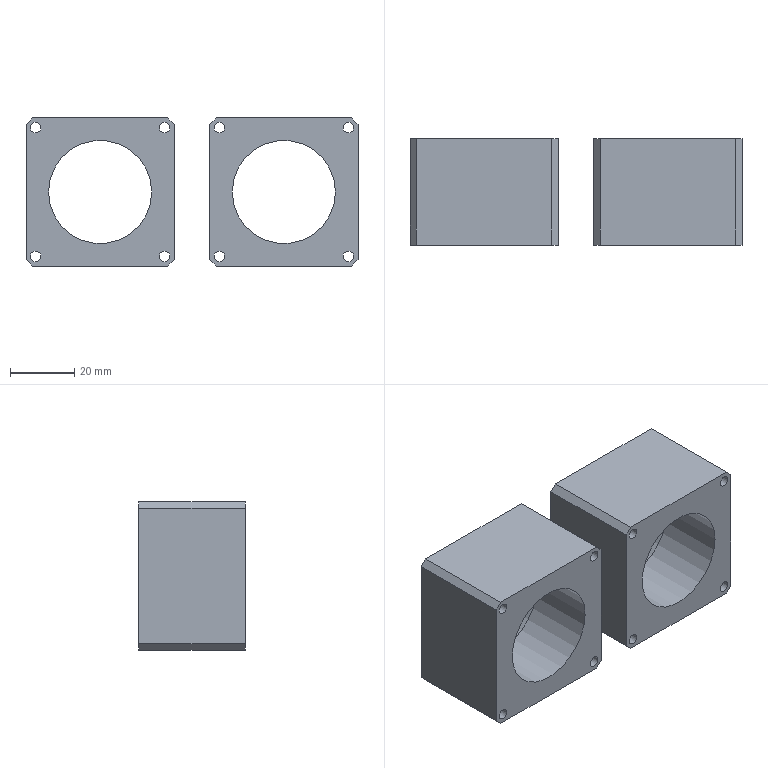CAM job | NX | 3+2 milling, drilling | part box 103 x 33 x 46 mm | stock box 108 x 35 x 51 mm
Tools:
number,name,description,diameter,corner_radius,flute_length,length,flutes
6,D6,平底铣刀-粗,6.0,0.0,25.0,75.0,2
9,D10,平底铣刀-粗,10.0,0.0,35.0,75.0,2
11,D4-J,平底铣刀-精,4.0,0.0,50.0,75.0,2
7,D6-J,平底铣刀-精,6.0,0.0,25.0,75.0,2
10,D10-J,平底铣刀-精,10.0,0.0,35.0,75.0,2
1,D80R0.8飞刀,圆鼻刀-粗,80.0,0.8,50.0,75.0,2
1,D80R0.8飞刀-J,圆鼻刀-精,80.0,0.8,50.0,75.0,2
2,D6倒角刀,倒角刀,6.0,0.0,3.0,25.0,2
20,M3X0.5,丝锥,2.5,0.0,35.0,50.0,2
12,ZT2.6,钻头,2.6,0.0,35.0,50.0,2
13,ZT3.4,钻头,3.4,0.0,35.0,50.0,2
Operations:
program,operation,operation_type,tool,method,geometry_group,spindle_rpm,surface_speed,feed_per_tooth,feed_cut,feed_plunge,cut_length_mm,path_length_mm,cut_time_min,machine_time_min
B,底壁铣飞面一刀开粗_COPY,VolumeBased25DMillingOperation,D80R0.8飞刀,分层开粗-切深K-步距G,W-B,2800.0,703.696,0.5357,3000.0,100.0,1267.165,2586.187,0.4224,0.5543
B,底壁铣飞面一刀精光_COPY,VolumeBased25DMillingOperation,D80R0.8飞刀-J,侧刃精光-切深K-步距G,W-B,4500.0,1130.973,0.1111,1000.0,100.0,210.998,306.998,0.211,0.2206
B,钻倒角_3,Operation,D6倒角刀,METHOD,W-B,8000.0,150.796,0.0625,1000.0,0.0,41.6,439.287,0.0416,0.0814
B,平面去毛刺6X45L_COPY,SurfaceContour,D6倒角刀,爬面_倒角-切深0-步距G,W-B,6500.0,122.519,0.1154,1500.0,100.0,639.96,1426.461,0.4266,0.5053
A,顶面,FaceMilling,D80R0.8飞刀,侧刃精光-切深K-步距G,W-A,4500.0,1385.0,0.1667,1500.0,100.0,197.0,293.0,0.1313,0.1409
A,外形粗_2,VolumeBased25DMillingOperation,D10,METHOD,W-A,8000.0,251.327,0.375,6000.0,80.0,18179.91,18500.41,3.03,3.062
A,型腔铣开粗-中_COPY,CavityMilling,D10,分层开粗-切深K-步距G,W-A,8000.0,251.32,0.25,4000.0,100.0,17009.688,18367.508,4.252,4.439
A,等高往复层切开粗-中_COPY,ZLevelMilling,D6,分层开粗-切深K-步距G,W-A,8000.0,150.792,0.1875,3000.0,100.0,1337.08,7446.112,0.4457,1.057
A,清角D4,ZLevelMilling,D4-J,METHOD,W-A,8000.0,100.531,0.125,2000.0,80.0,2773.694,3173.817,1.387,1.427
A,打点-深0.8,Operation,D6倒角刀,NONE,W-A,8000.0,150.796,0.0312,500.0,90.0,25.2,461.08,0.0504,0.094
A,通孔-M4螺纹底孔,Operation,ZT3.4,NONE,W-A,3000.0,31.102,0.05,300.0,90.0,312.0,965.121,1.04,1.105
A,盲锥孔-M3螺纹底孔,Operation,ZT2.6,NONE,W-A,3000.0,23.562,0.0167,100.0,90.0,84.0,447.614,0.84,0.8764
A,底精_1,VolumeBased25DMillingOperation,D6-J,METHOD,W-A,9000.0,169.646,0.0833,1500.0,100.0,654.533,957.033,0.4364,0.4666
A,底侧精_3,VolumeBased25DMillingOperation,D6-J,METHOD,W-A,9000.0,169.646,0.0833,1500.0,100.0,547.915,1073.685,0.3653,0.4179
A,仅选体,SurfaceContour,D6倒角刀,METHOD,W-A,8000.0,150.796,0.1875,3000.0,100.0,954.843,1825.194,0.3183,0.4053
A,钻倒角_1,Operation,D6倒角刀,METHOD,W-A,8000.0,150.796,0.0312,500.0,0.0,28.5,347.28,0.057,0.0889
A,钻倒角_2,Operation,D6倒角刀,METHOD,W-A,8000.0,150.796,0.0312,500.0,0.0,41.6,439.287,0.0832,0.123
A,盲锥孔-攻牙M3,Operation,M3X0.5,METHOD,W-A,1000.0,7.854,0.0003,0.5,90.0,60.0,399.614,120.0,120.034
A,底壁铣精光侧面-中_COPY,VolumeBased25DMillingOperation,D10-J,侧刃精光-切深K-步距G,W-A,8000.0,251.32,0.0625,1000.0,100.0,467.195,690.674,0.4672,0.4895
A,外形半精_2,VolumeBased25DMillingOperation,D10-J,METHOD,W-A,9000.0,169.646,0.0667,1200.0,100.0,1304.756,2245.106,1.087,1.181